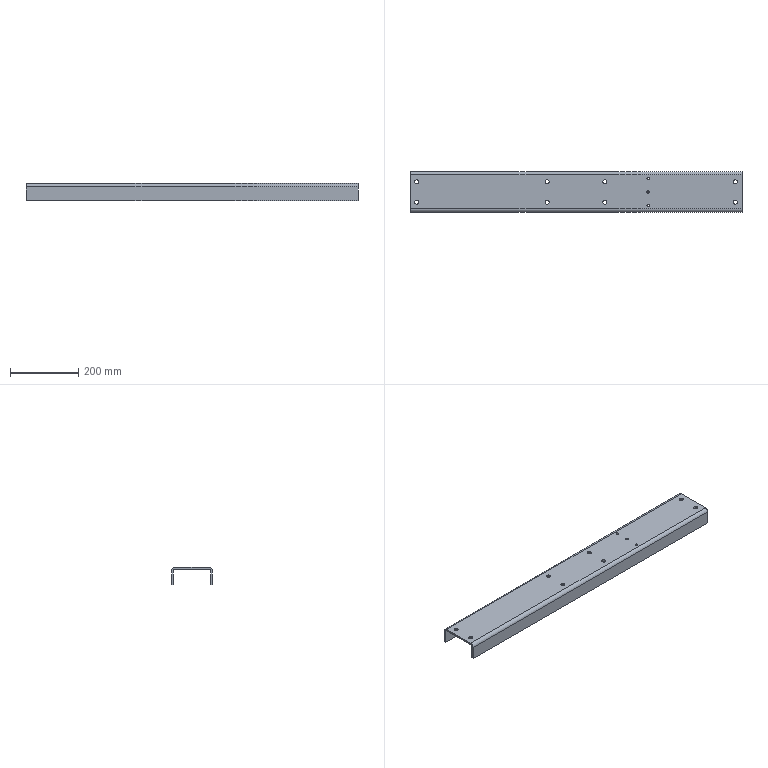Part | SolidWorks | features BaseBody 1 | 1 solid | 36 faces | box 976 x 120 x 50 mm | volume 988281 mm3 | cylinder 26 | plane 10 | commonest cylinder face diameters 12 x16 7 x6 10 x2 20 x2
STEP:
#1=CARTESIAN_POINT('',(-79.,30.,5.));
#2=VERTEX_POINT('',#1);
#3=CARTESIAN_POINT('',(-91.,30.,5.));
#4=VERTEX_POINT('',#3);
#5=CARTESIAN_POINT('',(-85.,30.,5.));
#6=DIRECTION('',(0.,0.,-1.));
#7=DIRECTION('',(-1.,0.,0.));
#8=AXIS2_PLACEMENT_3D('',#5,#6,#7);
#9=CIRCLE('',#8,6.);
#10=EDGE_CURVE('',#2,#4,#9,.T.);
#11=ORIENTED_EDGE('',*,*,#10,.F.);
#12=CARTESIAN_POINT('',(-79.,30.,0.));
#13=VERTEX_POINT('',#12);
#14=CARTESIAN_POINT('',(-79.,30.,5.));
#15=DIRECTION('',(0.,0.,-1.));
#16=VECTOR('',#15,1000.);
#17=LINE('',#14,#16);
#18=EDGE_CURVE('',#2,#13,#17,.T.);
#19=ORIENTED_EDGE('',*,*,#18,.T.);
#20=CARTESIAN_POINT('',(-91.,30.,0.));
#21=VERTEX_POINT('',#20);
#22=CARTESIAN_POINT('',(-85.,30.,0.));
#23=DIRECTION('',(0.,0.,-1.));
#24=DIRECTION('',(-1.,0.,0.));
#25=AXIS2_PLACEMENT_3D('',#22,#23,#24);
#26=CIRCLE('',#25,6.);
#27=EDGE_CURVE('',#13,#21,#26,.T.);
#28=ORIENTED_EDGE('',*,*,#27,.T.);
#29=CARTESIAN_POINT('',(-91.,30.,5.));
#30=DIRECTION('',(0.,0.,-1.));
#31=VECTOR('',#30,1000.);
#32=LINE('',#29,#31);
#33=EDGE_CURVE('',#4,#21,#32,.T.);
#34=ORIENTED_EDGE('',*,*,#33,.F.);
#35=EDGE_LOOP('',(#11,#19,#28,#34));
#36=FACE_OUTER_BOUND('',#35,.T.);
#37=CARTESIAN_POINT('',(-85.,30.,5.));
#38=DIRECTION('',(0.,0.,-1.));
#39=DIRECTION('',(-1.,0.,0.));
#40=AXIS2_PLACEMENT_3D('',#37,#38,#39);
#41=CYLINDRICAL_SURFACE('',#40,6.);
#42=ADVANCED_FACE('',(#36),#41,.F.);
#43=CARTESIAN_POINT('',(-79.,-30.,5.));
#44=VERTEX_POINT('',#43);
#45=CARTESIAN_POINT('',(-91.,-30.,5.));
#46=VERTEX_POINT('',#45);
#47=CARTESIAN_POINT('',(-85.,-30.,5.));
#48=DIRECTION('',(0.,0.,-1.));
#49=DIRECTION('',(-1.,0.,0.));
#50=AXIS2_PLACEMENT_3D('',#47,#48,#49);
#51=CIRCLE('',#50,6.);
#52=EDGE_CURVE('',#44,#46,#51,.T.);
#53=ORIENTED_EDGE('',*,*,#52,.F.);
#54=CARTESIAN_POINT('',(-79.,-30.,0.));
#55=VERTEX_POINT('',#54);
#56=CARTESIAN_POINT('',(-79.,-30.,5.));
#57=DIRECTION('',(0.,0.,-1.));
#58=VECTOR('',#57,1000.);
#59=LINE('',#56,#58);
#60=EDGE_CURVE('',#44,#55,#59,.T.);
#61=ORIENTED_EDGE('',*,*,#60,.T.);
#62=CARTESIAN_POINT('',(-91.,-30.,0.));
#63=VERTEX_POINT('',#62);
#64=CARTESIAN_POINT('',(-85.,-30.,0.));
#65=DIRECTION('',(0.,0.,-1.));
#66=DIRECTION('',(-1.,0.,0.));
#67=AXIS2_PLACEMENT_3D('',#64,#65,#66);
#68=CIRCLE('',#67,6.);
#69=EDGE_CURVE('',#55,#63,#68,.T.);
#70=ORIENTED_EDGE('',*,*,#69,.T.);
#71=CARTESIAN_POINT('',(-91.,-30.,5.));
#72=DIRECTION('',(0.,0.,-1.));
#73=VECTOR('',#72,1000.);
#74=LINE('',#71,#73);
#75=EDGE_CURVE('',#46,#63,#74,.T.);
#76=ORIENTED_EDGE('',*,*,#75,.F.);
#77=EDGE_LOOP('',(#53,#61,#70,#76));
#78=FACE_OUTER_BOUND('',#77,.T.);
#79=CARTESIAN_POINT('',(-85.,-30.,5.));
#80=DIRECTION('',(0.,0.,-1.));
#81=DIRECTION('',(-1.,0.,0.));
#82=AXIS2_PLACEMENT_3D('',#79,#80,#81);
#83=CYLINDRICAL_SURFACE('',#82,6.);
#84=ADVANCED_FACE('',(#78),#83,.F.);
#85=CARTESIAN_POINT('',(91.,30.,5.));
#86=VERTEX_POINT('',#85);
#87=CARTESIAN_POINT('',(79.,30.,5.));
#88=VERTEX_POINT('',#87);
#89=CARTESIAN_POINT('',(85.,30.,5.));
#90=DIRECTION('',(0.,0.,-1.));
#91=DIRECTION('',(-1.,0.,0.));
#92=AXIS2_PLACEMENT_3D('',#89,#90,#91);
#93=CIRCLE('',#92,6.);
#94=EDGE_CURVE('',#86,#88,#93,.T.);
#95=ORIENTED_EDGE('',*,*,#94,.F.);
#96=CARTESIAN_POINT('',(91.,30.,0.));
#97=VERTEX_POINT('',#96);
#98=CARTESIAN_POINT('',(91.,30.,5.));
#99=DIRECTION('',(0.,0.,-1.));
#100=VECTOR('',#99,1000.);
#101=LINE('',#98,#100);
#102=EDGE_CURVE('',#86,#97,#101,.T.);
#103=ORIENTED_EDGE('',*,*,#102,.T.);
#104=CARTESIAN_POINT('',(79.,30.,0.));
#105=VERTEX_POINT('',#104);
#106=CARTESIAN_POINT('',(85.,30.,0.));
#107=DIRECTION('',(0.,0.,-1.));
#108=DIRECTION('',(-1.,0.,0.));
#109=AXIS2_PLACEMENT_3D('',#106,#107,#108);
#110=CIRCLE('',#109,6.);
#111=EDGE_CURVE('',#97,#105,#110,.T.);
#112=ORIENTED_EDGE('',*,*,#111,.T.);
#113=CARTESIAN_POINT('',(79.,30.,5.));
#114=DIRECTION('',(0.,0.,-1.));
#115=VECTOR('',#114,1000.);
#116=LINE('',#113,#115);
#117=EDGE_CURVE('',#88,#105,#116,.T.);
#118=ORIENTED_EDGE('',*,*,#117,.F.);
#119=EDGE_LOOP('',(#95,#103,#112,#118));
#120=FACE_OUTER_BOUND('',#119,.T.);
#121=CARTESIAN_POINT('',(85.,30.,5.));
#122=DIRECTION('',(0.,0.,-1.));
#123=DIRECTION('',(-1.,0.,0.));
#124=AXIS2_PLACEMENT_3D('',#121,#122,#123);
#125=CYLINDRICAL_SURFACE('',#124,6.);
#126=ADVANCED_FACE('',(#120),#125,.F.);
#127=CARTESIAN_POINT('',(91.,-30.,5.));
#128=VERTEX_POINT('',#127);
#129=CARTESIAN_POINT('',(79.,-30.,5.));
#130=VERTEX_POINT('',#129);
#131=CARTESIAN_POINT('',(85.,-30.,5.));
#132=DIRECTION('',(0.,0.,-1.));
#133=DIRECTION('',(-1.,0.,0.));
#134=AXIS2_PLACEMENT_3D('',#131,#132,#133);
#135=CIRCLE('',#134,6.);
#136=EDGE_CURVE('',#128,#130,#135,.T.);
#137=ORIENTED_EDGE('',*,*,#136,.F.);
#138=CARTESIAN_POINT('',(91.,-30.,0.));
#139=VERTEX_POINT('',#138);
#140=CARTESIAN_POINT('',(91.,-30.,5.));
#141=DIRECTION('',(0.,0.,-1.));
#142=VECTOR('',#141,1000.);
#143=LINE('',#140,#142);
#144=EDGE_CURVE('',#128,#139,#143,.T.);
#145=ORIENTED_EDGE('',*,*,#144,.T.);
#146=CARTESIAN_POINT('',(79.,-30.,0.));
#147=VERTEX_POINT('',#146);
#148=CARTESIAN_POINT('',(85.,-30.,0.));
#149=DIRECTION('',(0.,0.,-1.));
#150=DIRECTION('',(-1.,0.,0.));
#151=AXIS2_PLACEMENT_3D('',#148,#149,#150);
#152=CIRCLE('',#151,6.);
#153=EDGE_CURVE('',#139,#147,#152,.T.);
#154=ORIENTED_EDGE('',*,*,#153,.T.);
#155=CARTESIAN_POINT('',(79.,-30.,5.));
#156=DIRECTION('',(0.,0.,-1.));
#157=VECTOR('',#156,1000.);
#158=LINE('',#155,#157);
#159=EDGE_CURVE('',#130,#147,#158,.T.);
#160=ORIENTED_EDGE('',*,*,#159,.F.);
#161=EDGE_LOOP('',(#137,#145,#154,#160));
#162=FACE_OUTER_BOUND('',#161,.T.);
#163=CARTESIAN_POINT('',(85.,-30.,5.));
#164=DIRECTION('',(0.,0.,-1.));
#165=DIRECTION('',(-1.,0.,0.));
#166=AXIS2_PLACEMENT_3D('',#163,#164,#165);
#167=CYLINDRICAL_SURFACE('',#166,6.);
#168=ADVANCED_FACE('',(#162),#167,.F.);
#169=CARTESIAN_POINT('',(215.5,40.,5.));
#170=VERTEX_POINT('',#169);
#171=CARTESIAN_POINT('',(208.5,40.,5.));
#172=VERTEX_POINT('',#171);
#173=CARTESIAN_POINT('',(212.,40.,5.));
#174=DIRECTION('',(0.,0.,-1.));
#175=DIRECTION('',(-1.,0.,0.));
#176=AXIS2_PLACEMENT_3D('',#173,#174,#175);
#177=CIRCLE('',#176,3.5);
#178=EDGE_CURVE('',#170,#172,#177,.T.);
#179=ORIENTED_EDGE('',*,*,#178,.F.);
#180=CARTESIAN_POINT('',(215.5,40.,0.));
#181=VERTEX_POINT('',#180);
#182=CARTESIAN_POINT('',(215.5,40.,5.));
#183=DIRECTION('',(0.,0.,-1.));
#184=VECTOR('',#183,1000.);
#185=LINE('',#182,#184);
#186=EDGE_CURVE('',#170,#181,#185,.T.);
#187=ORIENTED_EDGE('',*,*,#186,.T.);
#188=CARTESIAN_POINT('',(208.5,40.,0.));
#189=VERTEX_POINT('',#188);
#190=CARTESIAN_POINT('',(212.,40.,0.));
#191=DIRECTION('',(0.,0.,-1.));
#192=DIRECTION('',(-1.,0.,0.));
#193=AXIS2_PLACEMENT_3D('',#190,#191,#192);
#194=CIRCLE('',#193,3.5);
#195=EDGE_CURVE('',#181,#189,#194,.T.);
#196=ORIENTED_EDGE('',*,*,#195,.T.);
#197=CARTESIAN_POINT('',(208.5,40.,5.));
#198=DIRECTION('',(0.,0.,-1.));
#199=VECTOR('',#198,1000.);
#200=LINE('',#197,#199);
#201=EDGE_CURVE('',#172,#189,#200,.T.);
#202=ORIENTED_EDGE('',*,*,#201,.F.);
#203=EDGE_LOOP('',(#179,#187,#196,#202));
#204=FACE_OUTER_BOUND('',#203,.T.);
#205=CARTESIAN_POINT('',(212.,40.,5.));
#206=DIRECTION('',(0.,0.,-1.));
#207=DIRECTION('',(-1.,0.,0.));
#208=AXIS2_PLACEMENT_3D('',#205,#206,#207);
#209=CYLINDRICAL_SURFACE('',#208,3.5);
#210=ADVANCED_FACE('',(#204),#209,.F.);
#211=CARTESIAN_POINT('',(215.5,0.,5.));
#212=VERTEX_POINT('',#211);
#213=CARTESIAN_POINT('',(208.5,0.,5.));
#214=VERTEX_POINT('',#213);
#215=CARTESIAN_POINT('',(212.,0.,5.));
#216=DIRECTION('',(0.,0.,-1.));
#217=DIRECTION('',(-1.,0.,0.));
#218=AXIS2_PLACEMENT_3D('',#215,#216,#217);
#219=CIRCLE('',#218,3.5);
#220=EDGE_CURVE('',#212,#214,#219,.T.);
#221=ORIENTED_EDGE('',*,*,#220,.F.);
#222=CARTESIAN_POINT('',(215.5,0.,0.));
#223=VERTEX_POINT('',#222);
#224=CARTESIAN_POINT('',(215.5,0.,5.));
#225=DIRECTION('',(0.,0.,-1.));
#226=VECTOR('',#225,1000.);
#227=LINE('',#224,#226);
#228=EDGE_CURVE('',#212,#223,#227,.T.);
#229=ORIENTED_EDGE('',*,*,#228,.T.);
#230=CARTESIAN_POINT('',(208.5,0.,0.));
#231=VERTEX_POINT('',#230);
#232=CARTESIAN_POINT('',(212.,0.,0.));
#233=DIRECTION('',(0.,0.,-1.));
#234=DIRECTION('',(-1.,0.,0.));
#235=AXIS2_PLACEMENT_3D('',#232,#233,#234);
#236=CIRCLE('',#235,3.5);
#237=EDGE_CURVE('',#223,#231,#236,.T.);
#238=ORIENTED_EDGE('',*,*,#237,.T.);
#239=CARTESIAN_POINT('',(208.5,0.,5.));
#240=DIRECTION('',(0.,0.,-1.));
#241=VECTOR('',#240,1000.);
#242=LINE('',#239,#241);
#243=EDGE_CURVE('',#214,#231,#242,.T.);
#244=ORIENTED_EDGE('',*,*,#243,.F.);
#245=EDGE_LOOP('',(#221,#229,#238,#244));
#246=FACE_OUTER_BOUND('',#245,.T.);
#247=CARTESIAN_POINT('',(212.,0.,5.));
#248=DIRECTION('',(0.,0.,-1.));
#249=DIRECTION('',(-1.,0.,0.));
#250=AXIS2_PLACEMENT_3D('',#247,#248,#249);
#251=CYLINDRICAL_SURFACE('',#250,3.5);
#252=ADVANCED_FACE('',(#246),#251,.F.);
#253=CARTESIAN_POINT('',(215.5,-40.,5.));
#254=VERTEX_POINT('',#253);
#255=CARTESIAN_POINT('',(208.5,-40.,5.));
#256=VERTEX_POINT('',#255);
#257=CARTESIAN_POINT('',(212.,-40.,5.));
#258=DIRECTION('',(0.,0.,-1.));
#259=DIRECTION('',(-1.,0.,0.));
#260=AXIS2_PLACEMENT_3D('',#257,#258,#259);
#261=CIRCLE('',#260,3.5);
#262=EDGE_CURVE('',#254,#256,#261,.T.);
#263=ORIENTED_EDGE('',*,*,#262,.F.);
#264=CARTESIAN_POINT('',(215.5,-40.,0.));
#265=VERTEX_POINT('',#264);
#266=CARTESIAN_POINT('',(215.5,-40.,5.));
#267=DIRECTION('',(0.,0.,-1.));
#268=VECTOR('',#267,1000.);
#269=LINE('',#266,#268);
#270=EDGE_CURVE('',#254,#265,#269,.T.);
#271=ORIENTED_EDGE('',*,*,#270,.T.);
#272=CARTESIAN_POINT('',(208.5,-40.,0.));
#273=VERTEX_POINT('',#272);
#274=CARTESIAN_POINT('',(212.,-40.,0.));
#275=DIRECTION('',(0.,0.,-1.));
#276=DIRECTION('',(-1.,0.,0.));
#277=AXIS2_PLACEMENT_3D('',#274,#275,#276);
#278=CIRCLE('',#277,3.5);
#279=EDGE_CURVE('',#265,#273,#278,.T.);
#280=ORIENTED_EDGE('',*,*,#279,.T.);
#281=CARTESIAN_POINT('',(208.5,-40.,5.));
#282=DIRECTION('',(0.,0.,-1.));
#283=VECTOR('',#282,1000.);
#284=LINE('',#281,#283);
#285=EDGE_CURVE('',#256,#273,#284,.T.);
#286=ORIENTED_EDGE('',*,*,#285,.F.);
#287=EDGE_LOOP('',(#263,#271,#280,#286));
#288=FACE_OUTER_BOUND('',#287,.T.);
#289=CARTESIAN_POINT('',(212.,-40.,5.));
#290=DIRECTION('',(0.,0.,-1.));
#291=DIRECTION('',(-1.,0.,0.));
#292=AXIS2_PLACEMENT_3D('',#289,#290,#291);
#293=CYLINDRICAL_SURFACE('',#292,3.5);
#294=ADVANCED_FACE('',(#288),#293,.F.);
#295=CARTESIAN_POINT('',(-462.,30.,5.));
#296=VERTEX_POINT('',#295);
#297=CARTESIAN_POINT('',(-474.,30.,5.));
#298=VERTEX_POINT('',#297);
#299=CARTESIAN_POINT('',(-468.,30.,5.));
#300=DIRECTION('',(0.,0.,-1.));
#301=DIRECTION('',(-1.,0.,0.));
#302=AXIS2_PLACEMENT_3D('',#299,#300,#301);
#303=CIRCLE('',#302,6.);
#304=EDGE_CURVE('',#296,#298,#303,.T.);
#305=ORIENTED_EDGE('',*,*,#304,.F.);
#306=CARTESIAN_POINT('',(-462.,30.,0.));
#307=VERTEX_POINT('',#306);
#308=CARTESIAN_POINT('',(-462.,30.,5.));
#309=DIRECTION('',(0.,0.,-1.));
#310=VECTOR('',#309,1000.);
#311=LINE('',#308,#310);
#312=EDGE_CURVE('',#296,#307,#311,.T.);
#313=ORIENTED_EDGE('',*,*,#312,.T.);
#314=CARTESIAN_POINT('',(-474.,30.,0.));
#315=VERTEX_POINT('',#314);
#316=CARTESIAN_POINT('',(-468.,30.,0.));
#317=DIRECTION('',(0.,0.,-1.));
#318=DIRECTION('',(-1.,0.,0.));
#319=AXIS2_PLACEMENT_3D('',#316,#317,#318);
#320=CIRCLE('',#319,6.);
#321=EDGE_CURVE('',#307,#315,#320,.T.);
#322=ORIENTED_EDGE('',*,*,#321,.T.);
#323=CARTESIAN_POINT('',(-474.,30.,5.));
#324=DIRECTION('',(0.,0.,-1.));
#325=VECTOR('',#324,1000.);
#326=LINE('',#323,#325);
#327=EDGE_CURVE('',#298,#315,#326,.T.);
#328=ORIENTED_EDGE('',*,*,#327,.F.);
#329=EDGE_LOOP('',(#305,#313,#322,#328));
#330=FACE_OUTER_BOUND('',#329,.T.);
#331=CARTESIAN_POINT('',(-468.,30.,5.));
#332=DIRECTION('',(0.,0.,-1.));
#333=DIRECTION('',(-1.,0.,0.));
#334=AXIS2_PLACEMENT_3D('',#331,#332,#333);
#335=CYLINDRICAL_SURFACE('',#334,6.);
#336=ADVANCED_FACE('',(#330),#335,.F.);
#337=CARTESIAN_POINT('',(-462.,-30.,5.));
#338=VERTEX_POINT('',#337);
#339=CARTESIAN_POINT('',(-474.,-30.,5.));
#340=VERTEX_POINT('',#339);
#341=CARTESIAN_POINT('',(-468.,-30.,5.));
#342=DIRECTION('',(0.,0.,-1.));
#343=DIRECTION('',(-1.,0.,0.));
#344=AXIS2_PLACEMENT_3D('',#341,#342,#343);
#345=CIRCLE('',#344,6.);
#346=EDGE_CURVE('',#338,#340,#345,.T.);
#347=ORIENTED_EDGE('',*,*,#346,.F.);
#348=CARTESIAN_POINT('',(-462.,-30.,0.));
#349=VERTEX_POINT('',#348);
#350=CARTESIAN_POINT('',(-462.,-30.,5.));
#351=DIRECTION('',(0.,0.,-1.));
#352=VECTOR('',#351,1000.);
#353=LINE('',#350,#352);
#354=EDGE_CURVE('',#338,#349,#353,.T.);
#355=ORIENTED_EDGE('',*,*,#354,.T.);
#356=CARTESIAN_POINT('',(-474.,-30.,0.));
#357=VERTEX_POINT('',#356);
#358=CARTESIAN_POINT('',(-468.,-30.,0.));
#359=DIRECTION('',(0.,0.,-1.));
#360=DIRECTION('',(-1.,0.,0.));
#361=AXIS2_PLACEMENT_3D('',#358,#359,#360);
#362=CIRCLE('',#361,6.);
#363=EDGE_CURVE('',#349,#357,#362,.T.);
#364=ORIENTED_EDGE('',*,*,#363,.T.);
#365=CARTESIAN_POINT('',(-474.,-30.,5.));
#366=DIRECTION('',(0.,0.,-1.));
#367=VECTOR('',#366,1000.);
#368=LINE('',#365,#367);
#369=EDGE_CURVE('',#340,#357,#368,.T.);
#370=ORIENTED_EDGE('',*,*,#369,.F.);
#371=EDGE_LOOP('',(#347,#355,#364,#370));
#372=FACE_OUTER_BOUND('',#371,.T.);
#373=CARTESIAN_POINT('',(-468.,-30.,5.));
#374=DIRECTION('',(0.,0.,-1.));
#375=DIRECTION('',(-1.,0.,0.));
#376=AXIS2_PLACEMENT_3D('',#373,#374,#375);
#377=CYLINDRICAL_SURFACE('',#376,6.);
#378=ADVANCED_FACE('',(#372),#377,.F.);
#379=CARTESIAN_POINT('',(474.,30.,5.));
#380=VERTEX_POINT('',#379);
#381=CARTESIAN_POINT('',(462.,30.,5.));
#382=VERTEX_POINT('',#381);
#383=CARTESIAN_POINT('',(468.,30.,5.));
#384=DIRECTION('',(0.,0.,-1.));
#385=DIRECTION('',(-1.,0.,0.));
#386=AXIS2_PLACEMENT_3D('',#383,#384,#385);
#387=CIRCLE('',#386,6.);
#388=EDGE_CURVE('',#380,#382,#387,.T.);
#389=ORIENTED_EDGE('',*,*,#388,.F.);
#390=CARTESIAN_POINT('',(474.,30.,0.));
#391=VERTEX_POINT('',#390);
#392=CARTESIAN_POINT('',(474.,30.,5.));
#393=DIRECTION('',(0.,0.,-1.));
#394=VECTOR('',#393,1000.);
#395=LINE('',#392,#394);
#396=EDGE_CURVE('',#380,#391,#395,.T.);
#397=ORIENTED_EDGE('',*,*,#396,.T.);
#398=CARTESIAN_POINT('',(462.,30.,0.));
#399=VERTEX_POINT('',#398);
#400=CARTESIAN_POINT('',(468.,30.,0.));
#401=DIRECTION('',(0.,0.,-1.));
#402=DIRECTION('',(-1.,0.,0.));
#403=AXIS2_PLACEMENT_3D('',#400,#401,#402);
#404=CIRCLE('',#403,6.);
#405=EDGE_CURVE('',#391,#399,#404,.T.);
#406=ORIENTED_EDGE('',*,*,#405,.T.);
#407=CARTESIAN_POINT('',(462.,30.,5.));
#408=DIRECTION('',(0.,0.,-1.));
#409=VECTOR('',#408,1000.);
#410=LINE('',#407,#409);
#411=EDGE_CURVE('',#382,#399,#410,.T.);
#412=ORIENTED_EDGE('',*,*,#411,.F.);
#413=EDGE_LOOP('',(#389,#397,#406,#412));
#414=FACE_OUTER_BOUND('',#413,.T.);
#415=CARTESIAN_POINT('',(468.,30.,5.));
#416=DIRECTION('',(0.,0.,-1.));
#417=DIRECTION('',(-1.,0.,0.));
#418=AXIS2_PLACEMENT_3D('',#415,#416,#417);
#419=CYLINDRICAL_SURFACE('',#418,6.);
#420=ADVANCED_FACE('',(#414),#419,.F.);
#421=CARTESIAN_POINT('',(474.,-30.,5.));
#422=VERTEX_POINT('',#421);
#423=CARTESIAN_POINT('',(462.,-30.,5.));
#424=VERTEX_POINT('',#423);
#425=CARTESIAN_POINT('',(468.,-30.,5.));
#426=DIRECTION('',(0.,0.,-1.));
#427=DIRECTION('',(-1.,0.,0.));
#428=AXIS2_PLACEMENT_3D('',#425,#426,#427);
#429=CIRCLE('',#428,6.);
#430=EDGE_CURVE('',#422,#424,#429,.T.);
#431=ORIENTED_EDGE('',*,*,#430,.F.);
#432=CARTESIAN_POINT('',(474.,-30.,0.));
#433=VERTEX_POINT('',#432);
#434=CARTESIAN_POINT('',(474.,-30.,5.));
#435=DIRECTION('',(0.,0.,-1.));
#436=VECTOR('',#435,1000.);
#437=LINE('',#434,#436);
#438=EDGE_CURVE('',#422,#433,#437,.T.);
#439=ORIENTED_EDGE('',*,*,#438,.T.);
#440=CARTESIAN_POINT('',(462.,-30.,0.));
#441=VERTEX_POINT('',#440);
#442=CARTESIAN_POINT('',(468.,-30.,0.));
#443=DIRECTION('',(0.,0.,-1.));
#444=DIRECTION('',(-1.,0.,0.));
#445=AXIS2_PLACEMENT_3D('',#442,#443,#444);
#446=CIRCLE('',#445,6.);
#447=EDGE_CURVE('',#433,#441,#446,.T.);
#448=ORIENTED_EDGE('',*,*,#447,.T.);
#449=CARTESIAN_POINT('',(462.,-30.,5.));
#450=DIRECTION('',(0.,0.,-1.));
#451=VECTOR('',#450,1000.);
#452=LINE('',#449,#451);
#453=EDGE_CURVE('',#424,#441,#452,.T.);
#454=ORIENTED_EDGE('',*,*,#453,.F.);
#455=EDGE_LOOP('',(#431,#439,#448,#454));
#456=FACE_OUTER_BOUND('',#455,.T.);
#457=CARTESIAN_POINT('',(468.,-30.,5.));
#458=DIRECTION('',(0.,0.,-1.));
#459=DIRECTION('',(-1.,0.,0.));
#460=AXIS2_PLACEMENT_3D('',#457,#458,#459);
#461=CYLINDRICAL_SURFACE('',#460,6.);
#462=ADVANCED_FACE('',(#456),#461,.F.);
#463=CARTESIAN_POINT('',(-85.,30.,0.));
#464=DIRECTION('',(0.,0.,-1.));
#465=DIRECTION('',(-1.,0.,0.));
#466=AXIS2_PLACEMENT_3D('',#463,#464,#465);
#467=CIRCLE('',#466,6.);
#468=EDGE_CURVE('',#21,#13,#467,.T.);
#469=ORIENTED_EDGE('',*,*,#468,.F.);
#470=ORIENTED_EDGE('',*,*,#27,.F.);
#471=EDGE_LOOP('',(#469,#470));
#472=FACE_BOUND('',#471,.T.);
#473=CARTESIAN_POINT('',(-85.,-30.,0.));
#474=DIRECTION('',(0.,0.,-1.));
#475=DIRECTION('',(-1.,0.,0.));
#476=AXIS2_PLACEMENT_3D('',#473,#474,#475);
#477=CIRCLE('',#476,6.);
#478=EDGE_CURVE('',#63,#55,#477,.T.);
#479=ORIENTED_EDGE('',*,*,#478,.F.);
#480=ORIENTED_EDGE('',*,*,#69,.F.);
#481=EDGE_LOOP('',(#479,#480));
#482=FACE_BOUND('',#481,.T.);
#483=CARTESIAN_POINT('',(85.,30.,0.));
#484=DIRECTION('',(0.,0.,-1.));
#485=DIRECTION('',(-1.,0.,0.));
#486=AXIS2_PLACEMENT_3D('',#483,#484,#485);
#487=CIRCLE('',#486,6.);
#488=EDGE_CURVE('',#105,#97,#487,.T.);
#489=ORIENTED_EDGE('',*,*,#488,.F.);
#490=ORIENTED_EDGE('',*,*,#111,.F.);
#491=EDGE_LOOP('',(#489,#490));
#492=FACE_BOUND('',#491,.T.);
#493=CARTESIAN_POINT('',(85.,-30.,0.));
#494=DIRECTION('',(0.,0.,-1.));
#495=DIRECTION('',(-1.,0.,0.));
#496=AXIS2_PLACEMENT_3D('',#493,#494,#495);
#497=CIRCLE('',#496,6.);
#498=EDGE_CURVE('',#147,#139,#497,.T.);
#499=ORIENTED_EDGE('',*,*,#498,.F.);
#500=ORIENTED_EDGE('',*,*,#153,.F.);
#501=EDGE_LOOP('',(#499,#500));
#502=FACE_BOUND('',#501,.T.);
#503=CARTESIAN_POINT('',(212.,40.,0.));
#504=DIRECTION('',(0.,0.,-1.));
#505=DIRECTION('',(-1.,0.,0.));
#506=AXIS2_PLACEMENT_3D('',#503,#504,#505);
#507=CIRCLE('',#506,3.5);
#508=EDGE_CURVE('',#189,#181,#507,.T.);
#509=ORIENTED_EDGE('',*,*,#508,.F.);
#510=ORIENTED_EDGE('',*,*,#195,.F.);
#511=EDGE_LOOP('',(#509,#510));
#512=FACE_BOUND('',#511,.T.);
#513=CARTESIAN_POINT('',(212.,0.,0.));
#514=DIRECTION('',(0.,0.,-1.));
#515=DIRECTION('',(-1.,0.,0.));
#516=AXIS2_PLACEMENT_3D('',#513,#514,#515);
#517=CIRCLE('',#516,3.5);
#518=EDGE_CURVE('',#231,#223,#517,.T.);
#519=ORIENTED_EDGE('',*,*,#518,.F.);
#520=ORIENTED_EDGE('',*,*,#237,.F.);
#521=EDGE_LOOP('',(#519,#520));
#522=FACE_BOUND('',#521,.T.);
#523=CARTESIAN_POINT('',(212.,-40.,0.));
#524=DIRECTION('',(0.,0.,-1.));
#525=DIRECTION('',(-1.,0.,0.));
#526=AXIS2_PLACEMENT_3D('',#523,#524,#525);
#527=CIRCLE('',#526,3.5);
#528=EDGE_CURVE('',#273,#265,#527,.T.);
#529=ORIENTED_EDGE('',*,*,#528,.F.);
#530=ORIENTED_EDGE('',*,*,#279,.F.);
#531=EDGE_LOOP('',(#529,#530));
#532=FACE_BOUND('',#531,.T.);
#533=CARTESIAN_POINT('',(-468.,30.,0.));
#534=DIRECTION('',(0.,0.,-1.));
#535=DIRECTION('',(-1.,0.,0.));
#536=AXIS2_PLACEMENT_3D('',#533,#534,#535);
#537=CIRCLE('',#536,6.);
#538=EDGE_CURVE('',#315,#307,#537,.T.);
#539=ORIENTED_EDGE('',*,*,#538,.F.);
#540=ORIENTED_EDGE('',*,*,#321,.F.);
#541=EDGE_LOOP('',(#539,#540));
#542=FACE_BOUND('',#541,.T.);
#543=CARTESIAN_POINT('',(-468.,-30.,0.));
#544=DIRECTION('',(0.,0.,-1.));
#545=DIRECTION('',(-1.,0.,0.));
#546=AXIS2_PLACEMENT_3D('',#543,#544,#545);
#547=CIRCLE('',#546,6.);
#548=EDGE_CURVE('',#357,#349,#547,.T.);
#549=ORIENTED_EDGE('',*,*,#548,.F.);
#550=ORIENTED_EDGE('',*,*,#363,.F.);
#551=EDGE_LOOP('',(#549,#550));
#552=FACE_BOUND('',#551,.T.);
#553=CARTESIAN_POINT('',(468.,30.,0.));
#554=DIRECTION('',(0.,0.,-1.));
#555=DIRECTION('',(-1.,0.,0.));
#556=AXIS2_PLACEMENT_3D('',#553,#554,#555);
#557=CIRCLE('',#556,6.);
#558=EDGE_CURVE('',#399,#391,#557,.T.);
#559=ORIENTED_EDGE('',*,*,#558,.F.);
#560=ORIENTED_EDGE('',*,*,#405,.F.);
#561=EDGE_LOOP('',(#559,#560));
#562=FACE_BOUND('',#561,.T.);
#563=CARTESIAN_POINT('',(468.,-30.,0.));
#564=DIRECTION('',(0.,0.,-1.));
#565=DIRECTION('',(-1.,0.,0.));
#566=AXIS2_PLACEMENT_3D('',#563,#564,#565);
#567=CIRCLE('',#566,6.);
#568=EDGE_CURVE('',#441,#433,#567,.T.);
#569=ORIENTED_EDGE('',*,*,#568,.F.);
#570=ORIENTED_EDGE('',*,*,#447,.F.);
#571=EDGE_LOOP('',(#569,#570));
#572=FACE_BOUND('',#571,.T.);
#573=CARTESIAN_POINT('',(488.,-50.,0.));
#574=VERTEX_POINT('',#573);
#575=CARTESIAN_POINT('',(488.,50.,0.));
#576=VERTEX_POINT('',#575);
#577=CARTESIAN_POINT('',(488.,0.,0.));
#578=DIRECTION('',(0.,1.,0.));
#579=VECTOR('',#578,1000.);
#580=LINE('',#577,#579);
#581=EDGE_CURVE('',#574,#576,#580,.T.);
#582=ORIENTED_EDGE('',*,*,#581,.F.);
#583=CARTESIAN_POINT('',(-488.,-50.,0.));
#584=VERTEX_POINT('',#583);
#585=CARTESIAN_POINT('',(0.,-50.,0.));
#586=DIRECTION('',(1.,0.,0.));
#587=VECTOR('',#586,1000.);
#588=LINE('',#585,#587);
#589=EDGE_CURVE('',#584,#574,#588,.T.);
#590=ORIENTED_EDGE('',*,*,#589,.F.);
#591=CARTESIAN_POINT('',(-488.,50.,0.));
#592=VERTEX_POINT('',#591);
#593=CARTESIAN_POINT('',(-488.,0.,0.));
#594=DIRECTION('',(0.,-1.,0.));
#595=VECTOR('',#594,1000.);
#596=LINE('',#593,#595);
#597=EDGE_CURVE('',#592,#584,#596,.T.);
#598=ORIENTED_EDGE('',*,*,#597,.F.);
#599=CARTESIAN_POINT('',(0.,50.,0.));
#600=DIRECTION('',(-1.,0.,0.));
#601=VECTOR('',#600,1000.);
#602=LINE('',#599,#601);
#603=EDGE_CURVE('',#576,#592,#602,.T.);
#604=ORIENTED_EDGE('',*,*,#603,.F.);
#605=EDGE_LOOP('',(#582,#590,#598,#604));
#606=FACE_OUTER_BOUND('',#605,.T.);
#607=CARTESIAN_POINT('',(0.,0.,0.));
#608=DIRECTION('',(0.,0.,1.));
#609=DIRECTION('',(1.,0.,0.));
#610=AXIS2_PLACEMENT_3D('',#607,#608,#609);
#611=PLANE('',#610);
#612=ADVANCED_FACE('',(#472,#482,#492,#502,#512,#522,#532,#542,#552,#562,#572,#606),#611,.F.);
#613=ORIENTED_EDGE('',*,*,#18,.F.);
#614=CARTESIAN_POINT('',(-85.,30.,5.));
#615=DIRECTION('',(0.,0.,-1.));
#616=DIRECTION('',(-1.,0.,0.));
#617=AXIS2_PLACEMENT_3D('',#614,#615,#616);
#618=CIRCLE('',#617,6.);
#619=EDGE_CURVE('',#4,#2,#618,.T.);
#620=ORIENTED_EDGE('',*,*,#619,.F.);
#621=ORIENTED_EDGE('',*,*,#33,.T.);
#622=ORIENTED_EDGE('',*,*,#468,.T.);
#623=EDGE_LOOP('',(#613,#620,#621,#622));
#624=FACE_OUTER_BOUND('',#623,.T.);
#625=CARTESIAN_POINT('',(-85.,30.,5.));
#626=DIRECTION('',(0.,0.,-1.));
#627=DIRECTION('',(-1.,0.,0.));
#628=AXIS2_PLACEMENT_3D('',#625,#626,#627);
#629=CYLINDRICAL_SURFACE('',#628,6.);
#630=ADVANCED_FACE('',(#624),#629,.F.);
#631=ORIENTED_EDGE('',*,*,#60,.F.);
#632=CARTESIAN_POINT('',(-85.,-30.,5.));
#633=DIRECTION('',(0.,0.,-1.));
#634=DIRECTION('',(-1.,0.,0.));
#635=AXIS2_PLACEMENT_3D('',#632,#633,#634);
#636=CIRCLE('',#635,6.);
#637=EDGE_CURVE('',#46,#44,#636,.T.);
#638=ORIENTED_EDGE('',*,*,#637,.F.);
#639=ORIENTED_EDGE('',*,*,#75,.T.);
#640=ORIENTED_EDGE('',*,*,#478,.T.);
#641=EDGE_LOOP('',(#631,#638,#639,#640));
#642=FACE_OUTER_BOUND('',#641,.T.);
#643=CARTESIAN_POINT('',(-85.,-30.,5.));
#644=DIRECTION('',(0.,0.,-1.));
#645=DIRECTION('',(-1.,0.,0.));
#646=AXIS2_PLACEMENT_3D('',#643,#644,#645);
#647=CYLINDRICAL_SURFACE('',#646,6.);
#648=ADVANCED_FACE('',(#642),#647,.F.);
#649=ORIENTED_EDGE('',*,*,#102,.F.);
#650=CARTESIAN_POINT('',(85.,30.,5.));
#651=DIRECTION('',(0.,0.,-1.));
#652=DIRECTION('',(-1.,0.,0.));
#653=AXIS2_PLACEMENT_3D('',#650,#651,#652);
#654=CIRCLE('',#653,6.);
#655=EDGE_CURVE('',#88,#86,#654,.T.);
#656=ORIENTED_EDGE('',*,*,#655,.F.);
#657=ORIENTED_EDGE('',*,*,#117,.T.);
#658=ORIENTED_EDGE('',*,*,#488,.T.);
#659=EDGE_LOOP('',(#649,#656,#657,#658));
#660=FACE_OUTER_BOUND('',#659,.T.);
#661=CARTESIAN_POINT('',(85.,30.,5.));
#662=DIRECTION('',(0.,0.,-1.));
#663=DIRECTION('',(-1.,0.,0.));
#664=AXIS2_PLACEMENT_3D('',#661,#662,#663);
#665=CYLINDRICAL_SURFACE('',#664,6.);
#666=ADVANCED_FACE('',(#660),#665,.F.);
#667=ORIENTED_EDGE('',*,*,#144,.F.);
#668=CARTESIAN_POINT('',(85.,-30.,5.));
#669=DIRECTION('',(0.,0.,-1.));
#670=DIRECTION('',(-1.,0.,0.));
#671=AXIS2_PLACEMENT_3D('',#668,#669,#670);
#672=CIRCLE('',#671,6.);
#673=EDGE_CURVE('',#130,#128,#672,.T.);
#674=ORIENTED_EDGE('',*,*,#673,.F.);
#675=ORIENTED_EDGE('',*,*,#159,.T.);
#676=ORIENTED_EDGE('',*,*,#498,.T.);
#677=EDGE_LOOP('',(#667,#674,#675,#676));
#678=FACE_OUTER_BOUND('',#677,.T.);
#679=CARTESIAN_POINT('',(85.,-30.,5.));
#680=DIRECTION('',(0.,0.,-1.));
#681=DIRECTION('',(-1.,0.,0.));
#682=AXIS2_PLACEMENT_3D('',#679,#680,#681);
#683=CYLINDRICAL_SURFACE('',#682,6.);
#684=ADVANCED_FACE('',(#678),#683,.F.);
#685=ORIENTED_EDGE('',*,*,#186,.F.);
#686=CARTESIAN_POINT('',(212.,40.,5.));
#687=DIRECTION('',(0.,0.,-1.));
#688=DIRECTION('',(-1.,0.,0.));
#689=AXIS2_PLACEMENT_3D('',#686,#687,#688);
#690=CIRCLE('',#689,3.5);
#691=EDGE_CURVE('',#172,#170,#690,.T.);
#692=ORIENTED_EDGE('',*,*,#691,.F.);
#693=ORIENTED_EDGE('',*,*,#201,.T.);
#694=ORIENTED_EDGE('',*,*,#508,.T.);
#695=EDGE_LOOP('',(#685,#692,#693,#694));
#696=FACE_OUTER_BOUND('',#695,.T.);
#697=CARTESIAN_POINT('',(212.,40.,5.));
#698=DIRECTION('',(0.,0.,-1.));
#699=DIRECTION('',(-1.,0.,0.));
#700=AXIS2_PLACEMENT_3D('',#697,#698,#699);
#701=CYLINDRICAL_SURFACE('',#700,3.5);
#702=ADVANCED_FACE('',(#696),#701,.F.);
#703=ORIENTED_EDGE('',*,*,#228,.F.);
#704=CARTESIAN_POINT('',(212.,0.,5.));
#705=DIRECTION('',(0.,0.,-1.));
#706=DIRECTION('',(-1.,0.,0.));
#707=AXIS2_PLACEMENT_3D('',#704,#705,#706);
#708=CIRCLE('',#707,3.5);
#709=EDGE_CURVE('',#214,#212,#708,.T.);
#710=ORIENTED_EDGE('',*,*,#709,.F.);
#711=ORIENTED_EDGE('',*,*,#243,.T.);
#712=ORIENTED_EDGE('',*,*,#518,.T.);
#713=EDGE_LOOP('',(#703,#710,#711,#712));
#714=FACE_OUTER_BOUND('',#713,.T.);
#715=CARTESIAN_POINT('',(212.,0.,5.));
#716=DIRECTION('',(0.,0.,-1.));
#717=DIRECTION('',(-1.,0.,0.));
#718=AXIS2_PLACEMENT_3D('',#715,#716,#717);
#719=CYLINDRICAL_SURFACE('',#718,3.5);
#720=ADVANCED_FACE('',(#714),#719,.F.);
#721=ORIENTED_EDGE('',*,*,#270,.F.);
#722=CARTESIAN_POINT('',(212.,-40.,5.));
#723=DIRECTION('',(0.,0.,-1.));
#724=DIRECTION('',(-1.,0.,0.));
#725=AXIS2_PLACEMENT_3D('',#722,#723,#724);
#726=CIRCLE('',#725,3.5);
#727=EDGE_CURVE('',#256,#254,#726,.T.);
#728=ORIENTED_EDGE('',*,*,#727,.F.);
#729=ORIENTED_EDGE('',*,*,#285,.T.);
#730=ORIENTED_EDGE('',*,*,#528,.T.);
#731=EDGE_LOOP('',(#721,#728,#729,#730));
#732=FACE_OUTER_BOUND('',#731,.T.);
#733=CARTESIAN_POINT('',(212.,-40.,5.));
#734=DIRECTION('',(0.,0.,-1.));
#735=DIRECTION('',(-1.,0.,0.));
#736=AXIS2_PLACEMENT_3D('',#733,#734,#735);
#737=CYLINDRICAL_SURFACE('',#736,3.5);
#738=ADVANCED_FACE('',(#732),#737,.F.);
#739=ORIENTED_EDGE('',*,*,#312,.F.);
#740=CARTESIAN_POINT('',(-468.,30.,5.));
#741=DIRECTION('',(0.,0.,-1.));
#742=DIRECTION('',(-1.,0.,0.));
#743=AXIS2_PLACEMENT_3D('',#740,#741,#742);
#744=CIRCLE('',#743,6.);
#745=EDGE_CURVE('',#298,#296,#744,.T.);
#746=ORIENTED_EDGE('',*,*,#745,.F.);
#747=ORIENTED_EDGE('',*,*,#327,.T.);
#748=ORIENTED_EDGE('',*,*,#538,.T.);
#749=EDGE_LOOP('',(#739,#746,#747,#748));
#750=FACE_OUTER_BOUND('',#749,.T.);
#751=CARTESIAN_POINT('',(-468.,30.,5.));
#752=DIRECTION('',(0.,0.,-1.));
#753=DIRECTION('',(-1.,0.,0.));
#754=AXIS2_PLACEMENT_3D('',#751,#752,#753);
#755=CYLINDRICAL_SURFACE('',#754,6.);
#756=ADVANCED_FACE('',(#750),#755,.F.);
#757=ORIENTED_EDGE('',*,*,#354,.F.);
#758=CARTESIAN_POINT('',(-468.,-30.,5.));
#759=DIRECTION('',(0.,0.,-1.));
#760=DIRECTION('',(-1.,0.,0.));
#761=AXIS2_PLACEMENT_3D('',#758,#759,#760);
#762=CIRCLE('',#761,6.);
#763=EDGE_CURVE('',#340,#338,#762,.T.);
#764=ORIENTED_EDGE('',*,*,#763,.F.);
#765=ORIENTED_EDGE('',*,*,#369,.T.);
#766=ORIENTED_EDGE('',*,*,#548,.T.);
#767=EDGE_LOOP('',(#757,#764,#765,#766));
#768=FACE_OUTER_BOUND('',#767,.T.);
#769=CARTESIAN_POINT('',(-468.,-30.,5.));
#770=DIRECTION('',(0.,0.,-1.));
#771=DIRECTION('',(-1.,0.,0.));
#772=AXIS2_PLACEMENT_3D('',#769,#770,#771);
#773=CYLINDRICAL_SURFACE('',#772,6.);
#774=ADVANCED_FACE('',(#768),#773,.F.);
#775=ORIENTED_EDGE('',*,*,#396,.F.);
#776=CARTESIAN_POINT('',(468.,30.,5.));
#777=DIRECTION('',(0.,0.,-1.));
#778=DIRECTION('',(-1.,0.,0.));
#779=AXIS2_PLACEMENT_3D('',#776,#777,#778);
#780=CIRCLE('',#779,6.);
#781=EDGE_CURVE('',#382,#380,#780,.T.);
#782=ORIENTED_EDGE('',*,*,#781,.F.);
#783=ORIENTED_EDGE('',*,*,#411,.T.);
#784=ORIENTED_EDGE('',*,*,#558,.T.);
#785=EDGE_LOOP('',(#775,#782,#783,#784));
#786=FACE_OUTER_BOUND('',#785,.T.);
#787=CARTESIAN_POINT('',(468.,30.,5.));
#788=DIRECTION('',(0.,0.,-1.));
#789=DIRECTION('',(-1.,0.,0.));
#790=AXIS2_PLACEMENT_3D('',#787,#788,#789);
#791=CYLINDRICAL_SURFACE('',#790,6.);
#792=ADVANCED_FACE('',(#786),#791,.F.);
#793=ORIENTED_EDGE('',*,*,#438,.F.);
#794=CARTESIAN_POINT('',(468.,-30.,5.));
#795=DIRECTION('',(0.,0.,-1.));
#796=DIRECTION('',(-1.,0.,0.));
#797=AXIS2_PLACEMENT_3D('',#794,#795,#796);
#798=CIRCLE('',#797,6.);
#799=EDGE_CURVE('',#424,#422,#798,.T.);
#800=ORIENTED_EDGE('',*,*,#799,.F.);
#801=ORIENTED_EDGE('',*,*,#453,.T.);
#802=ORIENTED_EDGE('',*,*,#568,.T.);
#803=EDGE_LOOP('',(#793,#800,#801,#802));
#804=FACE_OUTER_BOUND('',#803,.T.);
#805=CARTESIAN_POINT('',(468.,-30.,5.));
#806=DIRECTION('',(0.,0.,-1.));
#807=DIRECTION('',(-1.,0.,0.));
#808=AXIS2_PLACEMENT_3D('',#805,#806,#807);
#809=CYLINDRICAL_SURFACE('',#808,6.);
#810=ADVANCED_FACE('',(#804),#809,.F.);
#811=ORIENTED_EDGE('',*,*,#603,.T.);
#812=CARTESIAN_POINT('',(-488.,55.,-5.));
#813=VERTEX_POINT('',#812);
#814=CARTESIAN_POINT('',(-488.,50.,-5.));
#815=DIRECTION('',(1.,0.,0.));
#816=DIRECTION('',(0.,0.,-1.));
#817=AXIS2_PLACEMENT_3D('',#814,#815,#816);
#818=CIRCLE('',#817,5.);
#819=EDGE_CURVE('',#813,#592,#818,.T.);
#820=ORIENTED_EDGE('',*,*,#819,.F.);
#821=CARTESIAN_POINT('',(488.,55.,-5.));
#822=VERTEX_POINT('',#821);
#823=CARTESIAN_POINT('',(-488.,55.,-5.));
#824=DIRECTION('',(-1.,0.,0.));
#825=VECTOR('',#824,1000.);
#826=LINE('',#823,#825);
#827=EDGE_CURVE('',#822,#813,#826,.T.);
#828=ORIENTED_EDGE('',*,*,#827,.F.);
#829=CARTESIAN_POINT('',(488.,50.,-5.));
#830=DIRECTION('',(-1.,0.,0.));
#831=DIRECTION('',(0.,0.,-1.));
#832=AXIS2_PLACEMENT_3D('',#829,#830,#831);
#833=CIRCLE('',#832,5.);
#834=EDGE_CURVE('',#576,#822,#833,.T.);
#835=ORIENTED_EDGE('',*,*,#834,.F.);
#836=EDGE_LOOP('',(#811,#820,#828,#835));
#837=FACE_OUTER_BOUND('',#836,.T.);
#838=CARTESIAN_POINT('',(-488.,50.,-5.));
#839=DIRECTION('',(1.,0.,0.));
#840=DIRECTION('',(0.,0.,-1.));
#841=AXIS2_PLACEMENT_3D('',#838,#839,#840);
#842=CYLINDRICAL_SURFACE('',#841,5.);
#843=ADVANCED_FACE('',(#837),#842,.F.);
#844=CARTESIAN_POINT('',(488.,-50.,5.));
#845=VERTEX_POINT('',#844);
#846=CARTESIAN_POINT('',(488.,50.,5.));
#847=VERTEX_POINT('',#846);
#848=CARTESIAN_POINT('',(488.,0.,5.));
#849=DIRECTION('',(0.,1.,0.));
#850=VECTOR('',#849,1000.);
#851=LINE('',#848,#850);
#852=EDGE_CURVE('',#845,#847,#851,.T.);
#853=ORIENTED_EDGE('',*,*,#852,.F.);
#854=CARTESIAN_POINT('',(488.,-60.,-5.));
#855=VERTEX_POINT('',#854);
#856=CARTESIAN_POINT('',(488.,-50.,-5.));
#857=DIRECTION('',(1.,0.,0.));
#858=DIRECTION('',(0.,0.,1.));
#859=AXIS2_PLACEMENT_3D('',#856,#857,#858);
#860=CIRCLE('',#859,10.);
#861=EDGE_CURVE('',#845,#855,#860,.T.);
#862=ORIENTED_EDGE('',*,*,#861,.T.);
#863=CARTESIAN_POINT('',(488.,-60.,-45.));
#864=VERTEX_POINT('',#863);
#865=CARTESIAN_POINT('',(488.,-60.,-25.));
#866=DIRECTION('',(0.,0.,-1.));
#867=VECTOR('',#866,1000.);
#868=LINE('',#865,#867);
#869=EDGE_CURVE('',#855,#864,#868,.T.);
#870=ORIENTED_EDGE('',*,*,#869,.T.);
#871=CARTESIAN_POINT('',(488.,-55.,-45.));
#872=VERTEX_POINT('',#871);
#873=CARTESIAN_POINT('',(488.,-57.5,-45.));
#874=DIRECTION('',(0.,1.,0.));
#875=VECTOR('',#874,1000.);
#876=LINE('',#873,#875);
#877=EDGE_CURVE('',#864,#872,#876,.T.);
#878=ORIENTED_EDGE('',*,*,#877,.T.);
#879=CARTESIAN_POINT('',(488.,-55.,-5.));
#880=VERTEX_POINT('',#879);
#881=CARTESIAN_POINT('',(488.,-55.,5.));
#882=DIRECTION('',(0.,0.,1.));
#883=VECTOR('',#882,1000.);
#884=LINE('',#881,#883);
#885=EDGE_CURVE('',#872,#880,#884,.T.);
#886=ORIENTED_EDGE('',*,*,#885,.T.);
#887=CARTESIAN_POINT('',(488.,-50.,-5.));
#888=DIRECTION('',(-1.,0.,0.));
#889=DIRECTION('',(0.,0.,1.));
#890=AXIS2_PLACEMENT_3D('',#887,#888,#889);
#891=CIRCLE('',#890,5.);
#892=EDGE_CURVE('',#880,#574,#891,.T.);
#893=ORIENTED_EDGE('',*,*,#892,.T.);
#894=ORIENTED_EDGE('',*,*,#581,.T.);
#895=ORIENTED_EDGE('',*,*,#834,.T.);
#896=CARTESIAN_POINT('',(488.,55.,-45.));
#897=VERTEX_POINT('',#896);
#898=CARTESIAN_POINT('',(488.,55.,5.));
#899=DIRECTION('',(0.,0.,-1.));
#900=VECTOR('',#899,1000.);
#901=LINE('',#898,#900);
#902=EDGE_CURVE('',#822,#897,#901,.T.);
#903=ORIENTED_EDGE('',*,*,#902,.T.);
#904=CARTESIAN_POINT('',(488.,60.,-45.));
#905=VERTEX_POINT('',#904);
#906=CARTESIAN_POINT('',(488.,57.5,-45.));
#907=DIRECTION('',(0.,1.,0.));
#908=VECTOR('',#907,1000.);
#909=LINE('',#906,#908);
#910=EDGE_CURVE('',#897,#905,#909,.T.);
#911=ORIENTED_EDGE('',*,*,#910,.T.);
#912=CARTESIAN_POINT('',(488.,60.,-5.));
#913=VERTEX_POINT('',#912);
#914=CARTESIAN_POINT('',(488.,60.,-25.));
#915=DIRECTION('',(0.,0.,1.));
#916=VECTOR('',#915,1000.);
#917=LINE('',#914,#916);
#918=EDGE_CURVE('',#905,#913,#917,.T.);
#919=ORIENTED_EDGE('',*,*,#918,.T.);
#920=CARTESIAN_POINT('',(488.,50.,-5.));
#921=DIRECTION('',(-1.,0.,0.));
#922=DIRECTION('',(0.,0.,-1.));
#923=AXIS2_PLACEMENT_3D('',#920,#921,#922);
#924=CIRCLE('',#923,10.);
#925=EDGE_CURVE('',#847,#913,#924,.T.);
#926=ORIENTED_EDGE('',*,*,#925,.F.);
#927=EDGE_LOOP('',(#853,#862,#870,#878,#886,#893,#894,#895,#903,#911,#919,#926));
#928=FACE_OUTER_BOUND('',#927,.T.);
#929=CARTESIAN_POINT('',(488.,0.,2.5));
#930=DIRECTION('',(-1.,0.,0.));
#931=DIRECTION('',(0.,0.,1.));
#932=AXIS2_PLACEMENT_3D('',#929,#930,#931);
#933=PLANE('',#932);
#934=ADVANCED_FACE('',(#928),#933,.F.);
#935=ORIENTED_EDGE('',*,*,#589,.T.);
#936=ORIENTED_EDGE('',*,*,#892,.F.);
#937=CARTESIAN_POINT('',(-488.,-55.,-5.));
#938=VERTEX_POINT('',#937);
#939=CARTESIAN_POINT('',(488.,-55.,-5.));
#940=DIRECTION('',(1.,0.,0.));
#941=VECTOR('',#940,1000.);
#942=LINE('',#939,#941);
#943=EDGE_CURVE('',#938,#880,#942,.T.);
#944=ORIENTED_EDGE('',*,*,#943,.F.);
#945=CARTESIAN_POINT('',(-488.,-50.,-5.));
#946=DIRECTION('',(1.,0.,0.));
#947=DIRECTION('',(0.,0.,1.));
#948=AXIS2_PLACEMENT_3D('',#945,#946,#947);
#949=CIRCLE('',#948,5.);
#950=EDGE_CURVE('',#584,#938,#949,.T.);
#951=ORIENTED_EDGE('',*,*,#950,.F.);
#952=EDGE_LOOP('',(#935,#936,#944,#951));
#953=FACE_OUTER_BOUND('',#952,.T.);
#954=CARTESIAN_POINT('',(488.,-50.,-5.));
#955=DIRECTION('',(-1.,0.,0.));
#956=DIRECTION('',(0.,0.,1.));
#957=AXIS2_PLACEMENT_3D('',#954,#955,#956);
#958=CYLINDRICAL_SURFACE('',#957,5.);
#959=ADVANCED_FACE('',(#953),#958,.F.);
#960=CARTESIAN_POINT('',(-488.,50.,5.));
#961=VERTEX_POINT('',#960);
#962=CARTESIAN_POINT('',(-488.,-50.,5.));
#963=VERTEX_POINT('',#962);
#964=CARTESIAN_POINT('',(-488.,0.,5.));
#965=DIRECTION('',(0.,-1.,0.));
#966=VECTOR('',#965,1000.);
#967=LINE('',#964,#966);
#968=EDGE_CURVE('',#961,#963,#967,.T.);
#969=ORIENTED_EDGE('',*,*,#968,.F.);
#970=CARTESIAN_POINT('',(-488.,60.,-5.));
#971=VERTEX_POINT('',#970);
#972=CARTESIAN_POINT('',(-488.,50.,-5.));
#973=DIRECTION('',(-1.,0.,0.));
#974=DIRECTION('',(0.,0.,-1.));
#975=AXIS2_PLACEMENT_3D('',#972,#973,#974);
#976=CIRCLE('',#975,10.);
#977=EDGE_CURVE('',#961,#971,#976,.T.);
#978=ORIENTED_EDGE('',*,*,#977,.T.);
#979=CARTESIAN_POINT('',(-488.,60.,-45.));
#980=VERTEX_POINT('',#979);
#981=CARTESIAN_POINT('',(-488.,60.,-25.));
#982=DIRECTION('',(0.,0.,-1.));
#983=VECTOR('',#982,1000.);
#984=LINE('',#981,#983);
#985=EDGE_CURVE('',#971,#980,#984,.T.);
#986=ORIENTED_EDGE('',*,*,#985,.T.);
#987=CARTESIAN_POINT('',(-488.,55.,-45.));
#988=VERTEX_POINT('',#987);
#989=CARTESIAN_POINT('',(-488.,57.5,-45.));
#990=DIRECTION('',(0.,-1.,0.));
#991=VECTOR('',#990,1000.);
#992=LINE('',#989,#991);
#993=EDGE_CURVE('',#980,#988,#992,.T.);
#994=ORIENTED_EDGE('',*,*,#993,.T.);
#995=CARTESIAN_POINT('',(-488.,55.,5.));
#996=DIRECTION('',(0.,0.,1.));
#997=VECTOR('',#996,1000.);
#998=LINE('',#995,#997);
#999=EDGE_CURVE('',#988,#813,#998,.T.);
#1000=ORIENTED_EDGE('',*,*,#999,.T.);
#1001=ORIENTED_EDGE('',*,*,#819,.T.);
#1002=ORIENTED_EDGE('',*,*,#597,.T.);
#1003=ORIENTED_EDGE('',*,*,#950,.T.);
#1004=CARTESIAN_POINT('',(-488.,-55.,-45.));
#1005=VERTEX_POINT('',#1004);
#1006=CARTESIAN_POINT('',(-488.,-55.,5.));
#1007=DIRECTION('',(0.,0.,-1.));
#1008=VECTOR('',#1007,1000.);
#1009=LINE('',#1006,#1008);
#1010=EDGE_CURVE('',#938,#1005,#1009,.T.);
#1011=ORIENTED_EDGE('',*,*,#1010,.T.);
#1012=CARTESIAN_POINT('',(-488.,-60.,-45.));
#1013=VERTEX_POINT('',#1012);
#1014=CARTESIAN_POINT('',(-488.,-57.5,-45.));
#1015=DIRECTION('',(0.,-1.,0.));
#1016=VECTOR('',#1015,1000.);
#1017=LINE('',#1014,#1016);
#1018=EDGE_CURVE('',#1005,#1013,#1017,.T.);
#1019=ORIENTED_EDGE('',*,*,#1018,.T.);
#1020=CARTESIAN_POINT('',(-488.,-60.,-5.));
#1021=VERTEX_POINT('',#1020);
#1022=CARTESIAN_POINT('',(-488.,-60.,-25.));
#1023=DIRECTION('',(0.,0.,1.));
#1024=VECTOR('',#1023,1000.);
#1025=LINE('',#1022,#1024);
#1026=EDGE_CURVE('',#1013,#1021,#1025,.T.);
#1027=ORIENTED_EDGE('',*,*,#1026,.T.);
#1028=CARTESIAN_POINT('',(-488.,-50.,-5.));
#1029=DIRECTION('',(1.,0.,0.));
#1030=DIRECTION('',(0.,0.,1.));
#1031=AXIS2_PLACEMENT_3D('',#1028,#1029,#1030);
#1032=CIRCLE('',#1031,10.);
#1033=EDGE_CURVE('',#963,#1021,#1032,.T.);
#1034=ORIENTED_EDGE('',*,*,#1033,.F.);
#1035=EDGE_LOOP('',(#969,#978,#986,#994,#1000,#1001,#1002,#1003,#1011,#1019,#1027,#1034));
#1036=FACE_OUTER_BOUND('',#1035,.T.);
#1037=CARTESIAN_POINT('',(-488.,0.,2.5));
#1038=DIRECTION('',(1.,0.,0.));
#1039=DIRECTION('',(0.,0.,-1.));
#1040=AXIS2_PLACEMENT_3D('',#1037,#1038,#1039);
#1041=PLANE('',#1040);
#1042=ADVANCED_FACE('',(#1036),#1041,.F.);
#1043=ORIENTED_EDGE('',*,*,#619,.T.);
#1044=ORIENTED_EDGE('',*,*,#10,.T.);
#1045=EDGE_LOOP('',(#1043,#1044));
#1046=FACE_BOUND('',#1045,.T.);
#1047=ORIENTED_EDGE('',*,*,#637,.T.);
#1048=ORIENTED_EDGE('',*,*,#52,.T.);
#1049=EDGE_LOOP('',(#1047,#1048));
#1050=FACE_BOUND('',#1049,.T.);
#1051=ORIENTED_EDGE('',*,*,#655,.T.);
#1052=ORIENTED_EDGE('',*,*,#94,.T.);
#1053=EDGE_LOOP('',(#1051,#1052));
#1054=FACE_BOUND('',#1053,.T.);
#1055=ORIENTED_EDGE('',*,*,#673,.T.);
#1056=ORIENTED_EDGE('',*,*,#136,.T.);
#1057=EDGE_LOOP('',(#1055,#1056));
#1058=FACE_BOUND('',#1057,.T.);
#1059=ORIENTED_EDGE('',*,*,#691,.T.);
#1060=ORIENTED_EDGE('',*,*,#178,.T.);
#1061=EDGE_LOOP('',(#1059,#1060));
#1062=FACE_BOUND('',#1061,.T.);
#1063=ORIENTED_EDGE('',*,*,#709,.T.);
#1064=ORIENTED_EDGE('',*,*,#220,.T.);
#1065=EDGE_LOOP('',(#1063,#1064));
#1066=FACE_BOUND('',#1065,.T.);
#1067=ORIENTED_EDGE('',*,*,#727,.T.);
#1068=ORIENTED_EDGE('',*,*,#262,.T.);
#1069=EDGE_LOOP('',(#1067,#1068));
#1070=FACE_BOUND('',#1069,.T.);
#1071=ORIENTED_EDGE('',*,*,#745,.T.);
#1072=ORIENTED_EDGE('',*,*,#304,.T.);
#1073=EDGE_LOOP('',(#1071,#1072));
#1074=FACE_BOUND('',#1073,.T.);
#1075=ORIENTED_EDGE('',*,*,#763,.T.);
#1076=ORIENTED_EDGE('',*,*,#346,.T.);
#1077=EDGE_LOOP('',(#1075,#1076));
#1078=FACE_BOUND('',#1077,.T.);
#1079=ORIENTED_EDGE('',*,*,#781,.T.);
#1080=ORIENTED_EDGE('',*,*,#388,.T.);
#1081=EDGE_LOOP('',(#1079,#1080));
#1082=FACE_BOUND('',#1081,.T.);
#1083=ORIENTED_EDGE('',*,*,#799,.T.);
#1084=ORIENTED_EDGE('',*,*,#430,.T.);
#1085=EDGE_LOOP('',(#1083,#1084));
#1086=FACE_BOUND('',#1085,.T.);
#1087=CARTESIAN_POINT('',(0.,50.,5.));
#1088=DIRECTION('',(-1.,0.,0.));
#1089=VECTOR('',#1088,1000.);
#1090=LINE('',#1087,#1089);
#1091=EDGE_CURVE('',#847,#961,#1090,.T.);
#1092=ORIENTED_EDGE('',*,*,#1091,.T.);
#1093=ORIENTED_EDGE('',*,*,#968,.T.);
#1094=CARTESIAN_POINT('',(0.,-50.,5.));
#1095=DIRECTION('',(1.,0.,0.));
#1096=VECTOR('',#1095,1000.);
#1097=LINE('',#1094,#1096);
#1098=EDGE_CURVE('',#963,#845,#1097,.T.);
#1099=ORIENTED_EDGE('',*,*,#1098,.T.);
#1100=ORIENTED_EDGE('',*,*,#852,.T.);
#1101=EDGE_LOOP('',(#1092,#1093,#1099,#1100));
#1102=FACE_OUTER_BOUND('',#1101,.T.);
#1103=CARTESIAN_POINT('',(0.,0.,5.));
#1104=DIRECTION('',(0.,0.,1.));
#1105=DIRECTION('',(1.,0.,0.));
#1106=AXIS2_PLACEMENT_3D('',#1103,#1104,#1105);
#1107=PLANE('',#1106);
#1108=ADVANCED_FACE('',(#1046,#1050,#1054,#1058,#1062,#1066,#1070,#1074,#1078,#1082,#1086,#1102),#1107,.T.);
#1109=ORIENTED_EDGE('',*,*,#999,.F.);
#1110=CARTESIAN_POINT('',(488.,55.,-45.));
#1111=DIRECTION('',(-1.,0.,0.));
#1112=VECTOR('',#1111,1000.);
#1113=LINE('',#1110,#1112);
#1114=EDGE_CURVE('',#897,#988,#1113,.T.);
#1115=ORIENTED_EDGE('',*,*,#1114,.F.);
#1116=ORIENTED_EDGE('',*,*,#902,.F.);
#1117=ORIENTED_EDGE('',*,*,#827,.T.);
#1118=EDGE_LOOP('',(#1109,#1115,#1116,#1117));
#1119=FACE_OUTER_BOUND('',#1118,.T.);
#1120=CARTESIAN_POINT('',(488.,55.,5.));
#1121=DIRECTION('',(0.,1.,0.));
#1122=DIRECTION('',(0.,0.,1.));
#1123=AXIS2_PLACEMENT_3D('',#1120,#1121,#1122);
#1124=PLANE('',#1123);
#1125=ADVANCED_FACE('',(#1119),#1124,.F.);
#1126=ORIENTED_EDGE('',*,*,#885,.F.);
#1127=CARTESIAN_POINT('',(-488.,-55.,-45.));
#1128=DIRECTION('',(1.,0.,0.));
#1129=VECTOR('',#1128,1000.);
#1130=LINE('',#1127,#1129);
#1131=EDGE_CURVE('',#1005,#872,#1130,.T.);
#1132=ORIENTED_EDGE('',*,*,#1131,.F.);
#1133=ORIENTED_EDGE('',*,*,#1010,.F.);
#1134=ORIENTED_EDGE('',*,*,#943,.T.);
#1135=EDGE_LOOP('',(#1126,#1132,#1133,#1134));
#1136=FACE_OUTER_BOUND('',#1135,.T.);
#1137=CARTESIAN_POINT('',(-488.,-55.,5.));
#1138=DIRECTION('',(0.,-1.,0.));
#1139=DIRECTION('',(0.,0.,-1.));
#1140=AXIS2_PLACEMENT_3D('',#1137,#1138,#1139);
#1141=PLANE('',#1140);
#1142=ADVANCED_FACE('',(#1136),#1141,.F.);
#1143=ORIENTED_EDGE('',*,*,#925,.T.);
#1144=CARTESIAN_POINT('',(-488.,60.,-5.));
#1145=DIRECTION('',(-1.,0.,0.));
#1146=VECTOR('',#1145,1000.);
#1147=LINE('',#1144,#1146);
#1148=EDGE_CURVE('',#913,#971,#1147,.T.);
#1149=ORIENTED_EDGE('',*,*,#1148,.T.);
#1150=ORIENTED_EDGE('',*,*,#977,.F.);
#1151=ORIENTED_EDGE('',*,*,#1091,.F.);
#1152=EDGE_LOOP('',(#1143,#1149,#1150,#1151));
#1153=FACE_OUTER_BOUND('',#1152,.T.);
#1154=CARTESIAN_POINT('',(-488.,50.,-5.));
#1155=DIRECTION('',(1.,0.,0.));
#1156=DIRECTION('',(0.,0.,-1.));
#1157=AXIS2_PLACEMENT_3D('',#1154,#1155,#1156);
#1158=CYLINDRICAL_SURFACE('',#1157,10.);
#1159=ADVANCED_FACE('',(#1153),#1158,.T.);
#1160=ORIENTED_EDGE('',*,*,#1033,.T.);
#1161=CARTESIAN_POINT('',(488.,-60.,-5.));
#1162=DIRECTION('',(1.,0.,0.));
#1163=VECTOR('',#1162,1000.);
#1164=LINE('',#1161,#1163);
#1165=EDGE_CURVE('',#1021,#855,#1164,.T.);
#1166=ORIENTED_EDGE('',*,*,#1165,.T.);
#1167=ORIENTED_EDGE('',*,*,#861,.F.);
#1168=ORIENTED_EDGE('',*,*,#1098,.F.);
#1169=EDGE_LOOP('',(#1160,#1166,#1167,#1168));
#1170=FACE_OUTER_BOUND('',#1169,.T.);
#1171=CARTESIAN_POINT('',(488.,-50.,-5.));
#1172=DIRECTION('',(-1.,0.,0.));
#1173=DIRECTION('',(0.,0.,1.));
#1174=AXIS2_PLACEMENT_3D('',#1171,#1172,#1173);
#1175=CYLINDRICAL_SURFACE('',#1174,10.);
#1176=ADVANCED_FACE('',(#1170),#1175,.T.);
#1177=ORIENTED_EDGE('',*,*,#993,.F.);
#1178=CARTESIAN_POINT('',(0.,60.,-45.));
#1179=DIRECTION('',(1.,0.,0.));
#1180=VECTOR('',#1179,1000.);
#1181=LINE('',#1178,#1180);
#1182=EDGE_CURVE('',#980,#905,#1181,.T.);
#1183=ORIENTED_EDGE('',*,*,#1182,.T.);
#1184=ORIENTED_EDGE('',*,*,#910,.F.);
#1185=ORIENTED_EDGE('',*,*,#1114,.T.);
#1186=EDGE_LOOP('',(#1177,#1183,#1184,#1185));
#1187=FACE_OUTER_BOUND('',#1186,.T.);
#1188=CARTESIAN_POINT('',(0.,57.5,-45.));
#1189=DIRECTION('',(0.,0.,-1.));
#1190=DIRECTION('',(-1.,0.,0.));
#1191=AXIS2_PLACEMENT_3D('',#1188,#1189,#1190);
#1192=PLANE('',#1191);
#1193=ADVANCED_FACE('',(#1187),#1192,.T.);
#1194=ORIENTED_EDGE('',*,*,#877,.F.);
#1195=CARTESIAN_POINT('',(0.,-60.,-45.));
#1196=DIRECTION('',(-1.,0.,0.));
#1197=VECTOR('',#1196,1000.);
#1198=LINE('',#1195,#1197);
#1199=EDGE_CURVE('',#864,#1013,#1198,.T.);
#1200=ORIENTED_EDGE('',*,*,#1199,.T.);
#1201=ORIENTED_EDGE('',*,*,#1018,.F.);
#1202=ORIENTED_EDGE('',*,*,#1131,.T.);
#1203=EDGE_LOOP('',(#1194,#1200,#1201,#1202));
#1204=FACE_OUTER_BOUND('',#1203,.T.);
#1205=CARTESIAN_POINT('',(0.,-57.5,-45.));
#1206=DIRECTION('',(0.,0.,-1.));
#1207=DIRECTION('',(-1.,0.,0.));
#1208=AXIS2_PLACEMENT_3D('',#1205,#1206,#1207);
#1209=PLANE('',#1208);
#1210=ADVANCED_FACE('',(#1204),#1209,.T.);
#1211=ORIENTED_EDGE('',*,*,#1148,.F.);
#1212=ORIENTED_EDGE('',*,*,#918,.F.);
#1213=ORIENTED_EDGE('',*,*,#1182,.F.);
#1214=ORIENTED_EDGE('',*,*,#985,.F.);
#1215=EDGE_LOOP('',(#1211,#1212,#1213,#1214));
#1216=FACE_OUTER_BOUND('',#1215,.T.);
#1217=CARTESIAN_POINT('',(488.,60.,5.));
#1218=DIRECTION('',(0.,1.,0.));
#1219=DIRECTION('',(0.,0.,1.));
#1220=AXIS2_PLACEMENT_3D('',#1217,#1218,#1219);
#1221=PLANE('',#1220);
#1222=ADVANCED_FACE('',(#1216),#1221,.T.);
#1223=ORIENTED_EDGE('',*,*,#1165,.F.);
#1224=ORIENTED_EDGE('',*,*,#1026,.F.);
#1225=ORIENTED_EDGE('',*,*,#1199,.F.);
#1226=ORIENTED_EDGE('',*,*,#869,.F.);
#1227=EDGE_LOOP('',(#1223,#1224,#1225,#1226));
#1228=FACE_OUTER_BOUND('',#1227,.T.);
#1229=CARTESIAN_POINT('',(-488.,-60.,5.));
#1230=DIRECTION('',(0.,-1.,0.));
#1231=DIRECTION('',(0.,0.,-1.));
#1232=AXIS2_PLACEMENT_3D('',#1229,#1230,#1231);
#1233=PLANE('',#1232);
#1234=ADVANCED_FACE('',(#1228),#1233,.T.);
#1235=CLOSED_SHELL('',(#42,#84,#126,#168,#210,#252,#294,#336,#378,#420,#462,#612,#630,#648,#666,#684,#702,#720,#738,#756,#774,#792,#810,#843,#934,#959,#1042,#1108,#1125,#1142,#1159,#1176,#1193,#1210,#1222,#1234));
#1236=MANIFOLD_SOLID_BREP('',#1235);
#1237=CARTESIAN_POINT('',(0.,0.,0.));
#1238=DIRECTION('',(0.,0.,1.));
#1239=DIRECTION('',(1.,0.,0.));
#1240=AXIS2_PLACEMENT_3D('',#1237,#1238,#1239);
#1241=(LENGTH_UNIT()NAMED_UNIT(*)SI_UNIT(.MILLI.,.METRE.));
#1242=UNCERTAINTY_MEASURE_WITH_UNIT(LENGTH_MEASURE(0.00001),#1241,'','');
#1243=(NAMED_UNIT(*)PLANE_ANGLE_UNIT()SI_UNIT($,.RADIAN.));
#1244=(NAMED_UNIT(*)SI_UNIT($,.STERADIAN.)SOLID_ANGLE_UNIT());
#1245=(GEOMETRIC_REPRESENTATION_CONTEXT(3)GLOBAL_UNCERTAINTY_ASSIGNED_CONTEXT((#1242))GLOBAL_UNIT_ASSIGNED_CONTEXT((#1241,#1243,#1244))REPRESENTATION_CONTEXT('',''));
#1246=ADVANCED_BREP_SHAPE_REPRESENTATION('',(#1236,#1240),#1245);